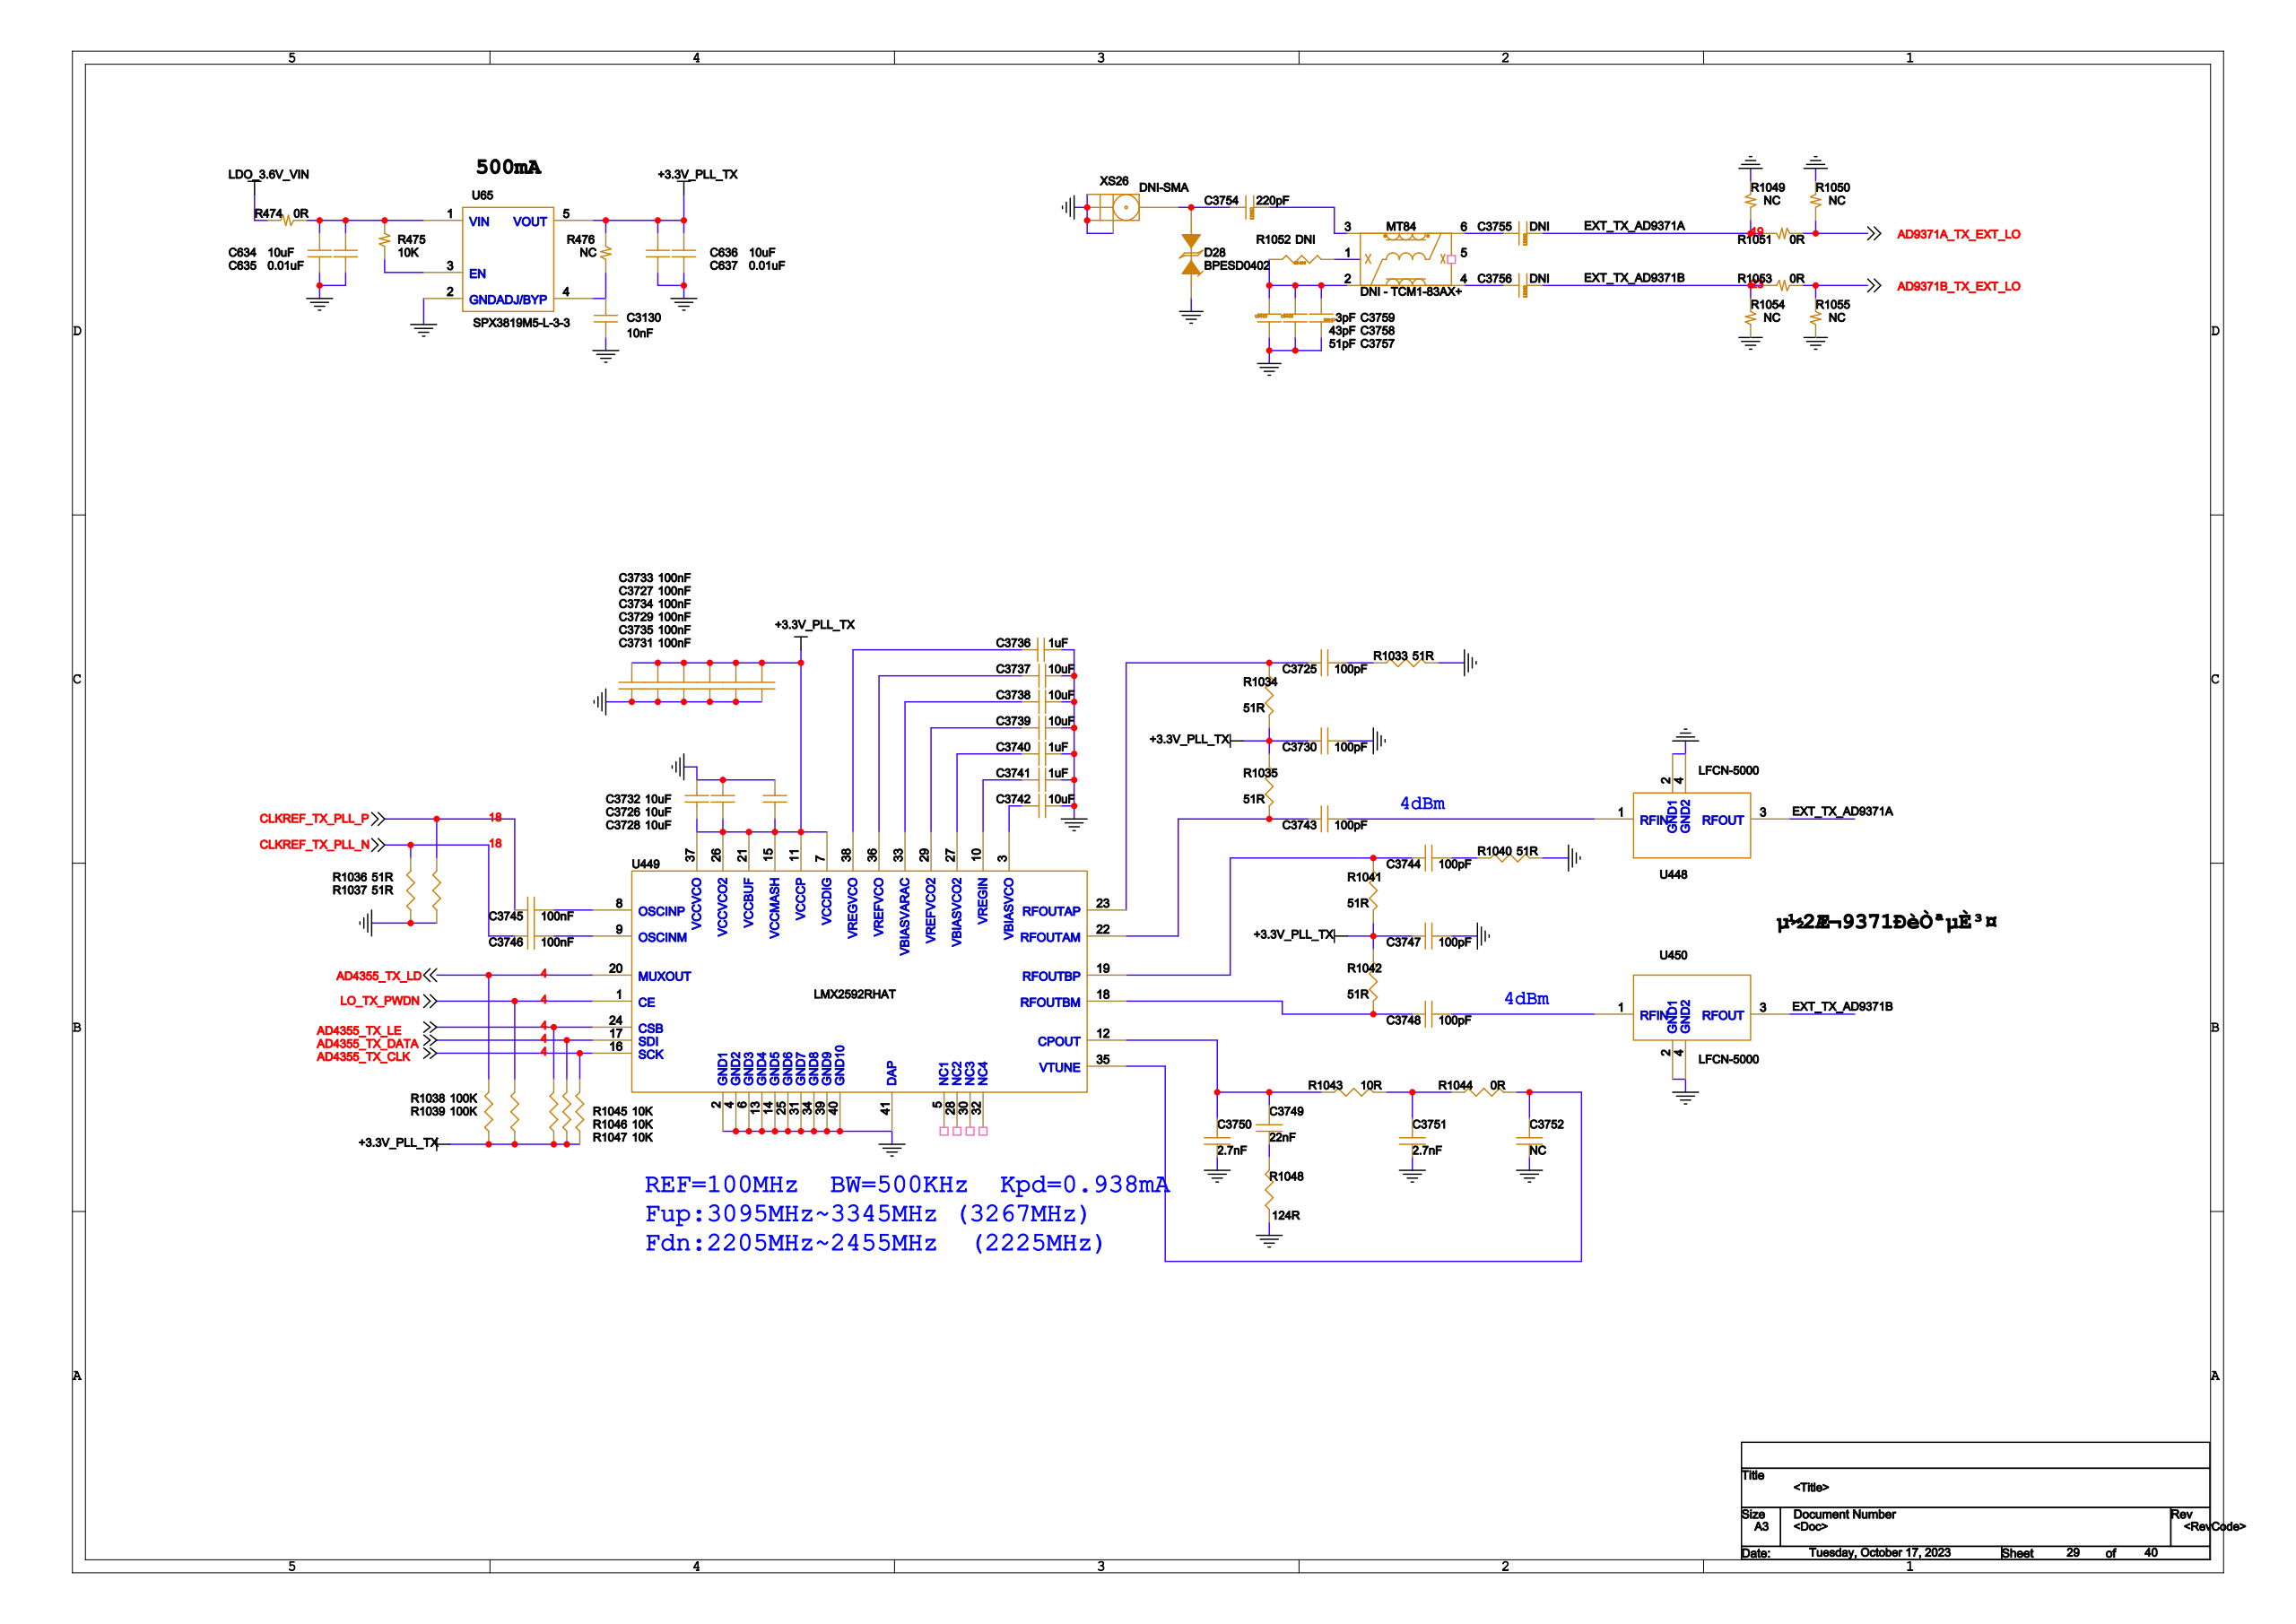Circuit board | Cadence Allegro | 1793 parts | 1223 nets | one sheet of the schematic
Parts on this sheet (reference | value | footprint):
C634 | 10uF | C0402
C635 | 0.01uF | C0402
C636 | 10uF | C0402
C637 | 0.01uF | C0402
C3130 | 10nF | C0402
C3725 | 100pF | C0402
C3726 | 10uF | C0402
C3727 | 100nF | C0402
C3728 | 10uF | C0402
C3729 | 100nF | C0402
C3730 | 100pF | C0402
C3731 | 100nF | C0402
C3732 | 10uF | C0402
C3733 | 100nF | C0402
C3734 | 100nF | C0402
C3735 | 100nF | C0402
C3736 | 1uF | C0402
C3737 | 10uF | C0402
C3738 | 10uF | C0402
C3739 | 10uF | C0402
C3740 | 1uF | C0402
C3741 | 1uF | C0402
C3742 | 10uF | C0402
C3743 | 100pF | C0402
C3744 | 100pF | C0402
C3745 | 100nF | C0402
C3746 | 100nF | C0402
C3747 | 100pF | C0402
C3748 | 100pF | C0402
C3749 | 22nF | C0402
C3750 | 2.7nF | C0402
C3751 | 2.7nF | C0402
C3752 | NC | C0402
C3754 | 220pF | C0402
C3755 | DNI | C0402
C3756 | DNI | C0402
C3757 | 51pF | C0402
C3758 | 43pF | C0402
C3759 | 3pF | C0402
D28 | BPESD0402 | C0402
MT84 | DNI - TCM1-83AX+ | TCM1-63AX
R474 | 0R | R0402
R475 | 10K | R0402
R476 | NC | R0402
R1033 | 51R | R0402
R1034 | 51R | R0402
R1035 | 51R | R0402
R1036 | 51R | R0402
R1037 | 51R | R0402
R1038 | 100K | R0402
R1039 | 100K | R0402
R1040 | 51R | R0402
R1041 | 51R | R0402
R1042 | 51R | R0402
R1043 | 10R | R0402
R1044 | 0R | R0402
R1045 | 10K | R0402
R1046 | 10K | R0402
R1047 | 10K | R0402
R1048 | 124R | R0402
R1049 | NC | R0402
R1050 | NC | R0402
R1051 | 0R | R0402
R1052 | DNI | R0402
R1053 | 0R | R0402
R1054 | NC | R0402
R1055 | NC | R0402
U65 | SPX3819M5-L-3-3 | SOT-23-5
U448 | LFCN-5000 | LFCN-3400
U449 | LMX2592RHAT | QFN-41-050P600X600X100
U450 | LFCN-5000 | LFCN-3400
XS26 | DNI-SMA | SMA_5X5MM
Nets of these parts (net: part-pin ...):
GND: C634-1 C635-1 C636-1 C637-1 C3130-1 C3726-1 C3727-1 C3728-1 C3729-1 C3730-2 C3731-1 C3732-1 C3733-1 C3734-1 C3735-1 C3736-2 C3737-1 C3738-1 C3739-1 C3740-1 C3741-1 C3742-1 C3747-2 C3750-1 C3751-1 C3752-1 C3757-2 C3758-2 C3759-1 D28-2 R1033-1 R1036-2 R1037-2 R1040-1 R1048-1 R1049-2 R1050-2 R1054-2 R1055-2 U65-2 U448-2 U448-4 U450-2 U450-4 XS26-2 XS26-3 XS26-4 XS26-5 U449-2 U449-4 U449-6 U449-13 U449-14 U449-25 U449-31 U449-34 U449-39 U449-40 U449-41
N17673343: C3754-2 D28-1 XS26-1
LDO_3.6V_VIN: R474-1
N17672813: C3743-2 U448-1
EXT_TX_AD9371A: C3755-1 R1049-1 R1051-1 U448-3
N17673064: C3748-2 U450-1
EXT_TX_AD9371B: C3756-1 R1053-1 R1054-1 U450-3
+3.3V_PLL_TX: C636-2 C637-2 C3726-2 C3727-2 C3728-2 C3729-2 C3730-1 C3731-2 C3732-2 C3733-2 C3734-2 C3735-2 C3747-1 R476-1 R1034-1 R1035-2 R1038-2 R1039-2 R1041-1 R1042-2 R1045-1 R1046-1 R1047-1 U65-5 U449-7 U449-11 U449-15 U449-21 U449-26 U449-37
N18037385: C3737-2 U449-36
N18037380: C3738-2 U449-33
N18037375: C3739-2 U449-29
N18037360: C3742-2 U449-3
N1578093: C634-2 C635-2 R474-2 R475-1 U65-1
N18037390: C3736-1 U449-38
N18037365: C3741-2 U449-10
N18037370: C3740-2 U449-27
N17673347: C3754-1 MT84-3
N17673361: C3755-2 MT84-6
N17673421: C3756-2 MT84-4
N17673386: MT84-1 R1052-1
N17673384: C3757-1 C3758-1 C3759-2 MT84-2 R1052-2
LO_TX_PWDN: R1039-1 U449-1
N17673109: C3749-2 C3750-2 R1043-1 U449-12
AD4355_TX_LE: R1045-2 U449-24
AD4355_TX_LD: R1038-1 U449-20
N17672993: C3746-2 U449-9
N17672958: C3745-2 U449-8
N17672807: C3743-1 R1035-1 U449-22
N17672469: C3725-1 R1034-2 U449-23
N17672868: C3744-1 R1041-2 U449-19
N17673043: C3748-1 R1042-1 U449-18
AD4355_TX_CLK: R1047-2 U449-16
AD4355_TX_DATA: R1046-2 U449-17
N17673123: C3752-2 R1044-2 U449-35
AD9371B_TX_EXT_LO: R1053-2 R1055-1
AD9371A_TX_EXT_LO: R1050-1 R1051-2
CLKREF_TX_PLL_P: C3745-1 R1037-1
CLKREF_TX_PLL_N: C3746-1 R1036-1
N17672475: C3725-2 R1033-2
N17672874: C3744-2 R1040-2
N17673117: C3751-2 R1043-2 R1044-1
N17673201: C3749-1 R1048-2
N1579505: C3130-2 R476-2 U65-4
N1578337: R475-2 U65-3